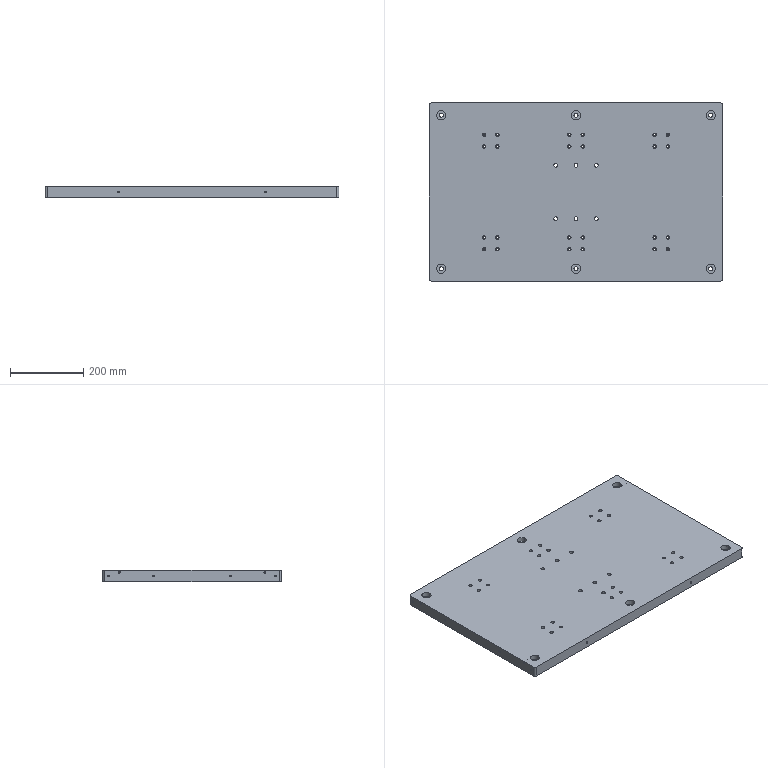NC program | Mastercam | posted with a generic post | part box 800 x 485 x 30 mm
Lines 631 to 1752 of 13355:
N6280 T20 M6
N6290 G0 G90 G17 G54 X332.781 Y6.265 A0. S5000 M3
N6300 G43 H20 Z50. M8
N6310 Z1.
N6320 G1 Z.533 F600.
N6330 Y17.265 Z.438 F4000.
N6340 Y28.265 Z.343
N6350 Y37.505 Z.264
N6360 X328.11 Y38.224 Z.249
N6370 X325. Y38.702 Z.221
N6380 X317.219 Y37.505 Z.154
N6390 Y36.679
N6400 Y25.679 Z.059
N6410 Y14.679 Z-.036
N6420 Y3.679 Z-.131
N6430 Y-.335 Z-.166
N6440 Y-7.321 Z-.226
N6450 Y-18.321 Z-.321
N6460 Y-29.321 Z-.416
N6470 Y-39.281 Z-.502
N6480 X321.887 Z-.511
N6490 X332.781 Z-.605
N6500 Y-37.758 Z-.606
N6510 Y-26.758 Z-.701
N6520 Y-15.758 Z-.796
N6530 Y-4.758 Z-.891
N6540 Y6.242 Z-.986
N6550 Y37.505
N6560 X325. Y38.702
N6570 X317.219 Y37.505
N6580 Y-.335
N6590 Y-39.281
N6600 X332.781
N6610 Y6.242
N6620 G2 X334.399 Y8.256 I2.063 J0.
N6630 G1 X344.186 Y10.416
N6640 G3 X345.804 Y12.43 I-.444 J2.014
N6650 G1 Y48.678
N6660 X325. Y51.878
N6670 X304.196 Y48.678
N6680 Y-.335
N6690 Y-52.304
N6700 X345.804
N6710 Y12.43
N6720 G2 X347.422 Y14.444 I2.063 J0.
N6730 G1 X357.209 Y16.603
N6740 G3 X358.827 Y18.617 I-.444 J2.014
N6750 G1 Y59.85
N6760 X325. Y65.054
N6770 X291.173 Y59.85
N6780 Y-.335
N6790 Y-65.327
N6800 X358.827
N6810 Y18.617
N6820 G2 X360.445 Y20.631 I2.063 J0.
N6830 G1 X370.232 Y22.791
N6840 G3 X371.85 Y24.805 I-.444 J2.014
N6850 G1 Y71.021
N6860 X325. Y78.231
N6870 X278.15 Y71.021
N6880 Y-.335
N6890 X278.151 Y-78.35
N6900 X371.849
N6910 X371.85 Y-78.347
N6920 Y24.805
N6930 G0 Z50.
N6940 X332.781 Y6.265
N6950 Z.014
N6960 G1 Z-.452 F600.
N6970 Y17.265 Z-.547 F4000.
N6980 Y28.265 Z-.642
N6990 Y37.505 Z-.722
N7000 X328.11 Y38.224 Z-.737
N7010 X325. Y38.702 Z-.764
N7020 X317.219 Y37.505 Z-.831
N7030 Y36.679 Z-.832
N7040 Y25.679 Z-.927
N7050 Y14.679 Z-1.022
N7060 Y3.679 Z-1.117
N7070 Y-.335 Z-1.152
N7080 Y-7.321 Z-1.212
N7090 Y-18.321 Z-1.307
N7100 Y-29.321 Z-1.402
N7110 Y-39.281 Z-1.488
N7120 X321.887 Z-1.497
N7130 X332.781 Z-1.591
N7140 Y-37.758 Z-1.592
N7150 Y-26.758 Z-1.687
N7160 Y-15.758 Z-1.782
N7170 Y-4.758 Z-1.876
N7180 Y6.242 Z-1.971
N7190 Y37.505
N7200 X325. Y38.702
N7210 X317.219 Y37.505
N7220 Y-.335
N7230 Y-39.281
N7240 X332.781
N7250 Y6.242
N7260 G2 X334.399 Y8.256 I2.063 J0.
N7270 G1 X344.186 Y10.416
N7280 G3 X345.804 Y12.43 I-.444 J2.014
N7290 G1 Y48.678
N7300 X325. Y51.878
N7310 X304.196 Y48.678
N7320 Y-.335
N7330 Y-52.304
N7340 X345.804
N7350 Y12.43
N7360 G2 X347.422 Y14.444 I2.063 J0.
N7370 G1 X357.209 Y16.603
N7380 G3 X358.827 Y18.617 I-.444 J2.014
N7390 G1 Y59.85
N7400 X325. Y65.054
N7410 X291.173 Y59.85
N7420 Y-.335
N7430 Y-65.327
N7440 X358.827
N7450 Y18.617
N7460 G2 X360.445 Y20.631 I2.063 J0.
N7470 G1 X370.232 Y22.791
N7480 G3 X371.85 Y24.805 I-.444 J2.014
N7490 G1 Y71.021
N7500 X325. Y78.231
N7510 X278.15 Y71.021
N7520 Y-.335
N7530 X278.151 Y-78.35
N7540 X371.849
N7550 X371.85 Y-78.347
N7560 Y24.805
N7570 G0 Z50.
N7580 X332.781 Y6.265
N7590 Z-.971
N7600 G1 Z-1.438 F600.
N7610 Y17.265 Z-1.533 F4000.
N7620 Y28.265 Z-1.628
N7630 Y37.505 Z-1.708
N7640 X328.11 Y38.224 Z-1.723
N7650 X325. Y38.702 Z-1.75
N7660 X317.219 Y37.505 Z-1.817
N7670 Y36.679 Z-1.818
N7680 Y25.679 Z-1.913
N7690 Y14.679 Z-2.008
N7700 Y3.679 Z-2.103
N7710 Y-.335 Z-2.137
N7720 Y-7.321 Z-2.198
N7730 Y-18.321 Z-2.293
N7740 Y-29.321 Z-2.388
N7750 Y-39.281 Z-2.473
N7760 X321.887 Z-2.482
N7770 X332.781 Z-2.576
N7780 Y-37.758 Z-2.577
N7790 Y-26.758 Z-2.672
N7800 Y-15.758 Z-2.767
N7810 Y-4.758 Z-2.862
N7820 Y6.242 Z-2.957
N7830 Y37.505
N7840 X325. Y38.702
N7850 X317.219 Y37.505
N7860 Y-.335
N7870 Y-39.281
N7880 X332.781
N7890 Y6.242
N7900 G2 X334.399 Y8.256 I2.063 J0.
N7910 G1 X344.186 Y10.416
N7920 G3 X345.804 Y12.43 I-.444 J2.014
N7930 G1 Y48.678
N7940 X325. Y51.878
N7950 X304.196 Y48.678
N7960 Y-.335
N7970 Y-52.304
N7980 X345.804
N7990 Y12.43
N8000 G2 X347.422 Y14.444 I2.063 J0.
N8010 G1 X357.209 Y16.603
N8020 G3 X358.827 Y18.617 I-.444 J2.014
N8030 G1 Y59.85
N8040 X325. Y65.054
N8050 X291.173 Y59.85
N8060 Y-.335
N8070 Y-65.327
N8080 X358.827
N8090 Y18.617
N8100 G2 X360.445 Y20.631 I2.063 J0.
N8110 G1 X370.232 Y22.791
N8120 G3 X371.85 Y24.805 I-.444 J2.014
N8130 G1 Y71.021
N8140 X325. Y78.231
N8150 X278.15 Y71.021
N8160 Y-.335
N8170 X278.151 Y-78.35
N8180 X371.849
N8190 X371.85 Y-78.347
N8200 Y24.805
N8210 G0 Z50.
N8220 X332.781 Y6.265
N8230 Z-1.957
N8240 G1 Z-2.424 F600.
N8250 Y17.265 Z-2.519 F4000.
N8260 Y28.265 Z-2.614
N8270 Y37.505 Z-2.693
N8280 X328.11 Y38.224 Z-2.709
N8290 X325. Y38.702 Z-2.736
N8300 X317.219 Y37.505 Z-2.803
N8310 Y36.679 Z-2.804
N8320 Y25.679 Z-2.899
N8330 Y14.679 Z-2.993
N8340 Y3.679 Z-3.088
N8350 Y-.335 Z-3.123
N8360 Y-7.321 Z-3.183
N8370 Y-18.321 Z-3.278
N8380 Y-29.321 Z-3.373
N8390 Y-39.281 Z-3.459
N8400 X321.887 Z-3.468
N8410 X332.781 Z-3.562
N8420 Y-37.758 Z-3.563
N8430 Y-26.758 Z-3.658
N8440 Y-15.758 Z-3.753
N8450 Y-4.758 Z-3.848
N8460 Y6.242 Z-3.943
N8470 Y37.505
N8480 X325. Y38.702
N8490 X317.219 Y37.505
N8500 Y-.335
N8510 Y-39.281
N8520 X332.781
N8530 Y6.242
N8540 G2 X334.399 Y8.256 I2.063 J0.
N8550 G1 X344.186 Y10.416
N8560 G3 X345.804 Y12.43 I-.444 J2.014
N8570 G1 Y48.678
N8580 X325. Y51.878
N8590 X304.196 Y48.678
N8600 Y-.335
N8610 Y-52.304
N8620 X345.804
N8630 Y12.43
N8640 G2 X347.422 Y14.444 I2.063 J0.
N8650 G1 X357.209 Y16.603
N8660 G3 X358.827 Y18.617 I-.444 J2.014
N8670 G1 Y59.85
N8680 X325. Y65.054
N8690 X291.173 Y59.85
N8700 Y-.335
N8710 Y-65.327
N8720 X358.827
N8730 Y18.617
N8740 G2 X360.445 Y20.631 I2.063 J0.
N8750 G1 X370.232 Y22.791
N8760 G3 X371.85 Y24.805 I-.444 J2.014
N8770 G1 Y71.021
N8780 X325. Y78.231
N8790 X278.15 Y71.021
N8800 Y-.335
N8810 X278.151 Y-78.35
N8820 X371.849
N8830 X371.85 Y-78.347
N8840 Y24.805
N8850 G0 Z50.
N8860 X332.781 Y6.265
N8870 Z-2.943
N8880 G1 Z-3.41 F600.
N8890 Y17.265 Z-3.504 F4000.
N8900 Y28.265 Z-3.599
N8910 Y37.505 Z-3.679
N8920 X328.11 Y38.224 Z-3.694
N8930 X325. Y38.702 Z-3.722
N8940 X317.219 Y37.505 Z-3.789
N8950 Y36.679
N8960 Y25.679 Z-3.884
N8970 Y14.679 Z-3.979
N8980 Y3.679 Z-4.074
N8990 Y-.335 Z-4.109
N9000 Y-7.321 Z-4.169
N9010 Y-18.321 Z-4.264
N9020 Y-29.321 Z-4.359
N9030 Y-39.281 Z-4.445
N9040 X321.887 Z-4.454
N9050 X332.781 Z-4.548
N9060 Y-37.758 Z-4.549
N9070 Y-26.758 Z-4.644
N9080 Y-15.758 Z-4.739
N9090 Y-4.758 Z-4.834
N9100 Y6.242 Z-4.929
N9110 Y37.505
N9120 X325. Y38.702
N9130 X317.219 Y37.505
N9140 Y-.335
N9150 Y-39.281
N9160 X332.781
N9170 Y6.242
N9180 G2 X334.399 Y8.256 I2.063 J0.
N9190 G1 X344.186 Y10.416
N9200 G3 X345.804 Y12.43 I-.444 J2.014
N9210 G1 Y48.678
N9220 X325. Y51.878
N9230 X304.196 Y48.678
N9240 Y-.335
N9250 Y-52.304
N9260 X345.804
N9270 Y12.43
N9280 G2 X347.422 Y14.444 I2.063 J0.
N9290 G1 X357.209 Y16.603
N9300 G3 X358.827 Y18.617 I-.444 J2.014
N9310 G1 Y59.85
N9320 X325. Y65.054
N9330 X291.173 Y59.85
N9340 Y-.335
N9350 Y-65.327
N9360 X358.827
N9370 Y18.617
N9380 G2 X360.445 Y20.631 I2.063 J0.
N9390 G1 X370.232 Y22.791
N9400 G3 X371.85 Y24.805 I-.444 J2.014
N9410 G1 Y71.021
N9420 X325. Y78.231
N9430 X278.15 Y71.021
N9440 Y-.335
N9450 X278.151 Y-78.35
N9460 X371.849
N9470 X371.85 Y-78.347
N9480 Y24.805
N9490 G0 Z50.
N9500 X332.781 Y6.265
N9510 Z-3.929
N9520 G1 Z-4.395 F600.
N9530 Y17.265 Z-4.49 F4000.
N9540 Y28.265 Z-4.585
N9550 Y37.505 Z-4.665
N9560 X328.11 Y38.224 Z-4.68
N9570 X325. Y38.702 Z-4.707
N9580 X317.219 Y37.505 Z-4.774
N9590 Y36.679 Z-4.775
N9600 Y25.679 Z-4.87
N9610 Y14.679 Z-4.965
N9620 Y3.679 Z-5.06
N9630 Y-.335 Z-5.094
N9640 Y-7.321 Z-5.155
N9650 Y-18.321 Z-5.25
N9660 Y-29.321 Z-5.345
N9670 Y-39.281 Z-5.431
N9680 X321.887 Z-5.44
N9690 X332.781 Z-5.534
N9700 Y-37.758 Z-5.535
N9710 Y-26.758 Z-5.629
N9720 Y-15.758 Z-5.724
N9730 Y-4.758 Z-5.819
N9740 Y6.242 Z-5.914
N9750 Y37.505
N9760 X325. Y38.702
N9770 X317.219 Y37.505
N9780 Y-.335
N9790 Y-39.281
N9800 X332.781
N9810 Y6.242
N9820 G2 X334.399 Y8.256 I2.063 J0.
N9830 G1 X344.186 Y10.416
N9840 G3 X345.804 Y12.43 I-.444 J2.014
N9850 G1 Y48.678
N9860 X325. Y51.878
N9870 X304.196 Y48.678
N9880 Y-.335
N9890 Y-52.304
N9900 X345.804
N9910 Y12.43
N9920 G2 X347.422 Y14.444 I2.063 J0.
N9930 G1 X357.209 Y16.603
N9940 G3 X358.827 Y18.617 I-.444 J2.014
N9950 G1 Y59.85
N9960 X325. Y65.054
N9970 X291.173 Y59.85
N9980 Y-.335
N9990 Y-65.327
N100 X358.827
N110 Y18.617
N120 G2 X360.445 Y20.631 I2.063 J0.
N130 G1 X370.232 Y22.791
N140 G3 X371.85 Y24.805 I-.444 J2.014
N150 G1 Y71.021
N160 X325. Y78.231
N170 X278.15 Y71.021
N180 Y-.335
N190 X278.151 Y-78.35
N200 X371.849
N210 X371.85 Y-78.347
N220 Y24.805
N230 G0 Z50.
N240 X332.781 Y6.265
N250 Z-4.914
N260 G1 Z-5.381 F600.
N270 Y17.265 Z-5.476 F4000.
N280 Y28.265 Z-5.571
N290 Y37.505 Z-5.651
N300 X328.11 Y38.224 Z-5.666
N310 X325. Y38.702 Z-5.693
N320 X317.219 Y37.505 Z-5.76
N330 Y36.679 Z-5.761
N340 Y25.679 Z-5.856
N350 Y14.679 Z-5.951
N360 Y3.679 Z-6.046
N370 Y-.335 Z-6.08
N380 Y-7.321 Z-6.14
N390 Y-18.321 Z-6.235
N400 Y-29.321 Z-6.33
N410 Y-39.281 Z-6.416
N420 X321.887 Z-6.425
N430 X332.781 Z-6.519
N440 Y-37.758 Z-6.52
N450 Y-26.758 Z-6.615
N460 Y-15.758 Z-6.71
N470 Y-4.758 Z-6.805
N480 Y6.242 Z-6.9
N490 Y37.505
N500 X325. Y38.702
N510 X317.219 Y37.505
N520 Y-.335
N530 Y-39.281
N540 X332.781
N550 Y6.242
N560 G2 X334.399 Y8.256 I2.063 J0.
N570 G1 X344.186 Y10.416
N580 G3 X345.804 Y12.43 I-.444 J2.014
N590 G1 Y48.678
N600 X325. Y51.878
N610 X304.196 Y48.678
N620 Y-.335
N630 Y-52.304
N640 X345.804
N650 Y12.43
N660 G2 X347.422 Y14.444 I2.063 J0.
N670 G1 X357.209 Y16.603
N680 G3 X358.827 Y18.617 I-.444 J2.014
N690 G1 Y59.85
N700 X325. Y65.054
N710 X291.173 Y59.85
N720 Y-.335
N730 Y-65.327
N740 X358.827
N750 Y18.617
N760 G2 X360.445 Y20.631 I2.063 J0.
N770 G1 X370.232 Y22.791
N780 G3 X371.85 Y24.805 I-.444 J2.014
N790 G1 Y71.021
N800 X325. Y78.231
N810 X278.15 Y71.021
N820 Y-.335
N830 X278.151 Y-78.35
N840 X371.849
N850 X371.85 Y-78.347
N860 Y24.805
N870 G0 Z50.
N880 X202.781 Y6.265
N890 Z1.
N900 G1 Z.533 F600.
N910 Y17.265 Z.438 F4000.
N920 Y28.265 Z.343
N930 Y37.505 Z.264
N940 X198.11 Y38.224 Z.249
N950 X195. Y38.702 Z.221
N960 X187.219 Y37.505 Z.154
N970 Y36.679
N980 Y25.679 Z.059
N990 Y14.679 Z-.036
N1000 Y3.679 Z-.131
N1010 Y-7.321 Z-.226
N1020 Y-18.321 Z-.321
N1030 Y-29.321 Z-.416
N1040 Y-39.281 Z-.502
N1050 X191.887 Z-.511
N1060 X202.781 Z-.605
N1070 Y-37.758 Z-.606
N1080 Y-26.758 Z-.701
N1090 Y-15.758 Z-.796
N1100 Y-4.758 Z-.891
N1110 Y-.335 Z-.929
N1120 Y6.242 Z-.986
N1130 Y37.505
N1140 X195. Y38.702
N1150 X187.219 Y37.505
N1160 Y-39.281
N1170 X202.781
N1180 Y-.335
N1190 Y6.242
N1200 G2 X204.399 Y8.256 I2.063 J0.
N1210 G1 X214.186 Y10.416
N1220 G3 X215.804 Y12.43 I-.444 J2.014
N1230 G1 Y48.678
N1240 X195. Y51.878
N1250 X174.196 Y48.678
N1260 Y-52.304
N1270 X215.804
N1280 Y-.335
N1290 Y12.43
N1300 G2 X217.422 Y14.444 I2.063 J0.
N1310 G1 X227.209 Y16.603
N1320 G3 X228.827 Y18.617 I-.444 J2.014
N1330 G1 Y59.85
N1340 X195. Y65.054
N1350 X161.173 Y59.85
N1360 Y-65.327
N1370 X228.827
N1380 Y-.335
N1390 Y18.617
N1400 G2 X230.445 Y20.631 I2.063 J0.
N1410 G1 X240.232 Y22.791
N1420 G3 X241.85 Y24.805 I-.444 J2.014
N1430 G1 Y71.021
N1440 X195. Y78.231
N1450 X148.15 Y71.021
N1460 Y-78.347
N1470 X148.151 Y-78.35
N1480 X241.849
N1490 X241.85 Y-.335
N1500 Y24.805
N1510 G0 Z50.
N1520 X202.781 Y6.265
N1530 Z.014
N1540 G1 Z-.452 F600.
N1550 Y17.265 Z-.547 F4000.
N1560 Y28.265 Z-.642
N1570 Y37.505 Z-.722
N1580 X198.11 Y38.224 Z-.737
N1590 X195. Y38.702 Z-.764
N1600 X187.219 Y37.505 Z-.831
N1610 Y36.679 Z-.832
N1620 Y25.679 Z-.927
N1630 Y14.679 Z-1.022
N1640 Y3.679 Z-1.117
N1650 Y-7.321 Z-1.212
N1660 Y-18.321 Z-1.307
N1670 Y-29.321 Z-1.402
N1680 Y-39.281 Z-1.488
N1690 X191.887 Z-1.497
N1700 X202.781 Z-1.591
N1710 Y-37.758 Z-1.592
N1720 Y-26.758 Z-1.687
N1730 Y-15.758 Z-1.782
N1740 Y-4.758 Z-1.876
N1750 Y-.335 Z-1.915
N1760 Y6.242 Z-1.971
N1770 Y37.505
N1780 X195. Y38.702
N1790 X187.219 Y37.505
N1800 Y-39.281
N1810 X202.781
N1820 Y-.335
N1830 Y6.242
N1840 G2 X204.399 Y8.256 I2.063 J0.
N1850 G1 X214.186 Y10.416
N1860 G3 X215.804 Y12.43 I-.444 J2.014
N1870 G1 Y48.678
N1880 X195. Y51.878
N1890 X174.196 Y48.678
N1900 Y-52.304
N1910 X215.804
N1920 Y-.335
N1930 Y12.43
N1940 G2 X217.422 Y14.444 I2.063 J0.
N1950 G1 X227.209 Y16.603
N1960 G3 X228.827 Y18.617 I-.444 J2.014
N1970 G1 Y59.85
N1980 X195. Y65.054
N1990 X161.173 Y59.85
N2000 Y-65.327
N2010 X228.827
N2020 Y-.335
N2030 Y18.617
N2040 G2 X230.445 Y20.631 I2.063 J0.
N2050 G1 X240.232 Y22.791
N2060 G3 X241.85 Y24.805 I-.444 J2.014
N2070 G1 Y71.021
N2080 X195. Y78.231
N2090 X148.15 Y71.021
N2100 Y-78.347
N2110 X148.151 Y-78.35
N2120 X241.849
N2130 X241.85 Y-.335
N2140 Y24.805
N2150 G0 Z50.
N2160 X202.781 Y6.265
N2170 Z-.971
N2180 G1 Z-1.438 F600.
N2190 Y17.265 Z-1.533 F4000.
N2200 Y28.265 Z-1.628
N2210 Y37.505 Z-1.708
N2220 X198.11 Y38.224 Z-1.723
N2230 X195. Y38.702 Z-1.75
N2240 X187.219 Y37.505 Z-1.817
N2250 Y36.679 Z-1.818
N2260 Y25.679 Z-1.913
N2270 Y14.679 Z-2.008
N2280 Y3.679 Z-2.103
N2290 Y-7.321 Z-2.198
N2300 Y-18.321 Z-2.293
N2310 Y-29.321 Z-2.388
N2320 Y-39.281 Z-2.473
N2330 X191.887 Z-2.482
N2340 X202.781 Z-2.576
N2350 Y-37.758 Z-2.577
N2360 Y-26.758 Z-2.672
N2370 Y-15.758 Z-2.767
N2380 Y-4.758 Z-2.862
N2390 Y-.335 Z-2.9
N2400 Y6.242 Z-2.957
N2410 Y37.505
N2420 X195. Y38.702
N2430 X187.219 Y37.505
N2440 Y-39.281
N2450 X202.781
N2460 Y-.335
N2470 Y6.242
N2480 G2 X204.399 Y8.256 I2.063 J0.
N2490 G1 X214.186 Y10.416
N2500 G3 X215.804 Y12.43 I-.444 J2.014
N2510 G1 Y48.678
N2520 X195. Y51.878
N2530 X174.196 Y48.678
N2540 Y-52.304
N2550 X215.804
N2560 Y-.335
N2570 Y12.43
N2580 G2 X217.422 Y14.444 I2.063 J0.
N2590 G1 X227.209 Y16.603
N2600 G3 X228.827 Y18.617 I-.444 J2.014
N2610 G1 Y59.85
N2620 X195. Y65.054
N2630 X161.173 Y59.85
N2640 Y-65.327
N2650 X228.827
N2660 Y-.335
N2670 Y18.617
N2680 G2 X230.445 Y20.631 I2.063 J0.
N2690 G1 X240.232 Y22.791
N2700 G3 X241.85 Y24.805 I-.444 J2.014
N2710 G1 Y71.021
N2720 X195. Y78.231
N2730 X148.15 Y71.021
N2740 Y-78.347
N2750 X148.151 Y-78.35
N2760 X241.849
N2770 X241.85 Y-.335
N2780 Y24.805
N2790 G0 Z50.
N2800 X202.781 Y6.265
N2810 Z-1.957
N2820 G1 Z-2.424 F600.
N2830 Y17.265 Z-2.519 F4000.
N2840 Y28.265 Z-2.614
N2850 Y37.505 Z-2.693
N2860 X198.11 Y38.224 Z-2.709
N2870 X195. Y38.702 Z-2.736
N2880 X187.219 Y37.505 Z-2.803
N2890 Y36.679 Z-2.804
N2900 Y25.679 Z-2.899
N2910 Y14.679 Z-2.993
N2920 Y3.679 Z-3.088
N2930 Y-7.321 Z-3.183
N2940 Y-18.321 Z-3.278
N2950 Y-29.321 Z-3.373
N2960 Y-39.281 Z-3.459
N2970 X191.887 Z-3.468
N2980 X202.781 Z-3.562
N2990 Y-37.758 Z-3.563
N3000 Y-26.758 Z-3.658
N3010 Y-15.758 Z-3.753
N3020 Y-4.758 Z-3.848
N3030 Y-.335 Z-3.886
N3040 Y6.242 Z-3.943
N3050 Y37.505
N3060 X195. Y38.702
N3070 X187.219 Y37.505
N3080 Y-39.281
N3090 X202.781
N3100 Y-.335
N3110 Y6.242
N3120 G2 X204.399 Y8.256 I2.063 J0.
N3130 G1 X214.186 Y10.416
N3140 G3 X215.804 Y12.43 I-.444 J2.014
N3150 G1 Y48.678
N3160 X195. Y51.878
N3170 X174.196 Y48.678
N3180 Y-52.304
N3190 X215.804
N3200 Y-.335
N3210 Y12.43
N3220 G2 X217.422 Y14.444 I2.063 J0.
N3230 G1 X227.209 Y16.603
N3240 G3 X228.827 Y18.617 I-.444 J2.014
N3250 G1 Y59.85
N3260 X195. Y65.054
N3270 X161.173 Y59.85
N3280 Y-65.327
N3290 X228.827
N3300 Y-.335
N3310 Y18.617
N3320 G2 X230.445 Y20.631 I2.063 J0.
N3330 G1 X240.232 Y22.791
N3340 G3 X241.85 Y24.805 I-.444 J2.014
N3350 G1 Y71.021
N3360 X195. Y78.231
N3370 X148.15 Y71.021
N3380 Y-78.347
N3390 X148.151 Y-78.35
N3400 X241.849
N3410 X241.85 Y-.335
N3420 Y24.805
N3430 G0 Z50.
N3440 X202.781 Y6.265
N3450 Z-2.943
N3460 G1 Z-3.41 F600.
N3470 Y17.265 Z-3.504 F4000.
N3480 Y28.265 Z-3.599
N3490 Y37.505 Z-3.679
N3500 X198.11 Y38.224 Z-3.694
N3510 X195. Y38.702 Z-3.722
N3520 X187.219 Y37.505 Z-3.789
N3530 Y36.679
N3540 Y25.679 Z-3.884
N3550 Y14.679 Z-3.979
N3560 Y3.679 Z-4.074
N3570 Y-7.321 Z-4.169
N3580 Y-18.321 Z-4.264
N3590 Y-29.321 Z-4.359
N3600 Y-39.281 Z-4.445
N3610 X191.887 Z-4.454
N3620 X202.781 Z-4.548
N3630 Y-37.758 Z-4.549
N3640 Y-26.758 Z-4.644
N3650 Y-15.758 Z-4.739
N3660 Y-4.758 Z-4.834
N3670 Y-.335 Z-4.872
N3680 Y6.242 Z-4.929
N3690 Y37.505
N3700 X195. Y38.702
N3710 X187.219 Y37.505
N3720 Y-39.281
N3730 X202.781
N3740 Y-.335
N3750 Y6.242
N3760 G2 X204.399 Y8.256 I2.063 J0.
N3770 G1 X214.186 Y10.416
N3780 G3 X215.804 Y12.43 I-.444 J2.014
N3790 G1 Y48.678
N3800 X195. Y51.878
N3810 X174.196 Y48.678
N3820 Y-52.304
N3830 X215.804
N3840 Y-.335
N3850 Y12.43
N3860 G2 X217.422 Y14.444 I2.063 J0.
N3870 G1 X227.209 Y16.603
N3880 G3 X228.827 Y18.617 I-.444 J2.014
N3890 G1 Y59.85
N3900 X195. Y65.054
N3910 X161.173 Y59.85
N3920 Y-65.327
N3930 X228.827
N3940 Y-.335
N3950 Y18.617
N3960 G2 X230.445 Y20.631 I2.063 J0.
N3970 G1 X240.232 Y22.791
N3980 G3 X241.85 Y24.805 I-.444 J2.014
N3990 G1 Y71.021
N4000 X195. Y78.231
N4010 X148.15 Y71.021
N4020 Y-78.347
N4030 X148.151 Y-78.35
N4040 X241.849
N4050 X241.85 Y-.335
N4060 Y24.805
N4070 G0 Z50.
N4080 X202.781 Y6.265
N4090 Z-3.929
N4100 G1 Z-4.395 F600.
N4110 Y17.265 Z-4.49 F4000.
N4120 Y28.265 Z-4.585
N4130 Y37.505 Z-4.665
N4140 X198.11 Y38.224 Z-4.68
N4150 X195. Y38.702 Z-4.707
N4160 X187.219 Y37.505 Z-4.774
N4170 Y36.679 Z-4.775
N4180 Y25.679 Z-4.87
N4190 Y14.679 Z-4.965
N4200 Y3.679 Z-5.06
N4210 Y-7.321 Z-5.155
N4220 Y-18.321 Z-5.25
N4230 Y-29.321 Z-5.345
N4240 Y-39.281 Z-5.431
N4250 X191.887 Z-5.44
N4260 X202.781 Z-5.534
N4270 Y-37.758 Z-5.535
N4280 Y-26.758 Z-5.629
N4290 Y-15.758 Z-5.724
N4300 Y-4.758 Z-5.819
N4310 Y-.335 Z-5.858
N4320 Y6.242 Z-5.914
N4330 Y37.505
N4340 X195. Y38.702
N4350 X187.219 Y37.505
N4360 Y-39.281
N4370 X202.781
N4380 Y-.335
N4390 Y6.242
N4400 G2 X204.399 Y8.256 I2.063 J0.
N4410 G1 X214.186 Y10.416
N4420 G3 X215.804 Y12.43 I-.444 J2.014
N4430 G1 Y48.678
N4440 X195. Y51.878
N4450 X174.196 Y48.678
N4460 Y-52.304
N4470 X215.804
N4480 Y-.335
N4490 Y12.43
N4500 G2 X217.422 Y14.444 I2.063 J0.
N4510 G1 X227.209 Y16.603
N4520 G3 X228.827 Y18.617 I-.444 J2.014
N4530 G1 Y59.85
N4540 X195. Y65.054
N4550 X161.173 Y59.85
N4560 Y-65.327
N4570 X228.827
N4580 Y-.335
N4590 Y18.617
N4600 G2 X230.445 Y20.631 I2.063 J0.
N4610 G1 X240.232 Y22.791
N4620 G3 X241.85 Y24.805 I-.444 J2.014
N4630 G1 Y71.021
N4640 X195. Y78.231
N4650 X148.15 Y71.021
N4660 Y-78.347
N4670 X148.151 Y-78.35
N4680 X241.849
N4690 X241.85 Y-.335
N4700 Y24.805
N4710 G0 Z50.
N4720 X202.781 Y6.265
N4730 Z-4.914
N4740 G1 Z-5.381 F600.
N4750 Y17.265 Z-5.476 F4000.
N4760 Y28.265 Z-5.571
N4770 Y37.505 Z-5.651
N4780 X198.11 Y38.224 Z-5.666
N4790 X195. Y38.702 Z-5.693
N4800 X187.219 Y37.505 Z-5.76
N4810 Y36.679 Z-5.761
N4820 Y25.679 Z-5.856
N4830 Y14.679 Z-5.951
N4840 Y3.679 Z-6.046
N4850 Y-7.321 Z-6.14
N4860 Y-18.321 Z-6.235
N4870 Y-29.321 Z-6.33
N4880 Y-39.281 Z-6.416
N4890 X191.887 Z-6.425
N4900 X202.781 Z-6.519
N4910 Y-37.758 Z-6.52
N4920 Y-26.758 Z-6.615
N4930 Y-15.758 Z-6.71
N4940 Y-4.758 Z-6.805
N4950 Y-.335 Z-6.843
N4960 Y6.242 Z-6.9
N4970 Y37.505
N4980 X195. Y38.702
N4990 X187.219 Y37.505
N5000 Y-39.281
N5010 X202.781
N5020 Y-.335
N5030 Y6.242
N5040 G2 X204.399 Y8.256 I2.063 J0.
N5050 G1 X214.186 Y10.416
N5060 G3 X215.804 Y12.43 I-.444 J2.014
N5070 G1 Y48.678
N5080 X195. Y51.878
N5090 X174.196 Y48.678
N5100 Y-52.304
N5110 X215.804
N5120 Y-.335
N5130 Y12.43
N5140 G2 X217.422 Y14.444 I2.063 J0.
N5150 G1 X227.209 Y16.603
N5160 G3 X228.827 Y18.617 I-.444 J2.014
N5170 G1 Y59.85
N5180 X195. Y65.054
N5190 X161.173 Y59.85
N5200 Y-65.327
N5210 X228.827
N5220 Y-.335
N5230 Y18.617
N5240 G2 X230.445 Y20.631 I2.063 J0.
N5250 G1 X240.232 Y22.791
N5260 G3 X241.85 Y24.805 I-.444 J2.014
N5270 G1 Y71.021
N5280 X195. Y78.231
N5290 X148.15 Y71.021
N5300 Y-78.347
N5310 X148.151 Y-78.35
N5320 X241.849
N5330 X241.85 Y-.335
N5340 Y24.805
N5350 G0 Z50.
N5360 X72.781 Y6.265
N5370 Z1.
N5380 G1 Z.533 F600.
N5390 Y17.265 Z.438 F4000.
N5400 Y28.265 Z.343
N5410 Y37.505 Z.264
N5420 X68.11 Y38.224 Z.249
N5430 X65. Y38.702 Z.221
N5440 X57.219 Y37.505 Z.154
N5450 Y36.679
N5460 Y25.679 Z.059
N5470 Y14.679 Z-.036
N5480 Y3.679 Z-.131
N5490 Y-7.321 Z-.226
N5500 Y-18.321 Z-.321
N5510 Y-29.321 Z-.416
N5520 Y-39.281 Z-.502
N5530 X61.887 Z-.511
N5540 X72.781 Z-.605
N5550 Y-37.758 Z-.606
N5560 Y-26.758 Z-.701
N5570 Y-15.758 Z-.796
N5580 Y-4.758 Z-.891
N5590 Y-.335 Z-.929
N5600 Y6.242 Z-.986
N5610 Y37.505
N5620 X65. Y38.702
N5630 X57.219 Y37.505
N5640 Y-39.281
N5650 X72.781
N5660 Y-.335
N5670 Y6.242
N5680 G2 X74.399 Y8.256 I2.063 J0.
N5690 G1 X84.186 Y10.416
N5700 G3 X85.804 Y12.43 I-.444 J2.014
N5710 G1 Y48.678
N5720 X65. Y51.878
N5730 X44.196 Y48.678
N5740 Y-52.304
N5750 X85.804
N5760 Y-.335
N5770 Y12.43
N5780 G2 X87.422 Y14.444 I2.063 J0.
N5790 G1 X97.209 Y16.603
N5800 G3 X98.827 Y18.617 I-.444 J2.014
N5810 G1 Y59.85
N5820 X65. Y65.054
N5830 X31.173 Y59.85
N5840 Y-65.327
N5850 X98.827
N5860 Y-.335
N5870 Y18.617
N5880 G2 X100.445 Y20.631 I2.063 J0.
N5890 G1 X110.232 Y22.791
N5900 G3 X111.85 Y24.805 I-.444 J2.014
N5910 G1 Y71.021
N5920 X65. Y78.231
N5930 X18.15 Y71.021
N5940 Y-78.347
N5950 X18.151 Y-78.35
N5960 X111.849
N5970 X111.85 Y-.335
N5980 Y24.805
N5990 G0 Z50.
N6000 X72.781 Y6.265
N6010 Z.014
N6020 G1 Z-.452 F600.
N6030 Y17.265 Z-.547 F4000.
N6040 Y28.265 Z-.642
N6050 Y37.505 Z-.722
N6060 X68.11 Y38.224 Z-.737
N6070 X65. Y38.702 Z-.764
N6080 X57.219 Y37.505 Z-.831
N6090 Y36.679 Z-.832
N6100 Y25.679 Z-.927
N6110 Y14.679 Z-1.022
N6120 Y3.679 Z-1.117
N6130 Y-7.321 Z-1.212
N6140 Y-18.321 Z-1.307
N6150 Y-29.321 Z-1.402
N6160 Y-39.281 Z-1.488
N6170 X61.887 Z-1.497
N6180 X72.781 Z-1.591
N6190 Y-37.758 Z-1.592
N6200 Y-26.758 Z-1.687
N6210 Y-15.758 Z-1.782
N6220 Y-4.758 Z-1.876
N6230 Y-.335 Z-1.915
N6240 Y6.242 Z-1.971
N6250 Y37.505
N6260 X65. Y38.702
N6270 X57.219 Y37.505
N6280 Y-39.281
N6290 X72.781
N6300 Y-.335
N6310 Y6.242
N6320 G2 X74.399 Y8.256 I2.063 J0.
N6330 G1 X84.186 Y10.416
N6340 G3 X85.804 Y12.43 I-.444 J2.014
N6350 G1 Y48.678
N6360 X65. Y51.878
N6370 X44.196 Y48.678
N6380 Y-52.304
N6390 X85.804
N6400 Y-.335
N6410 Y12.43
N6420 G2 X87.422 Y14.444 I2.063 J0.
N6430 G1 X97.209 Y16.603
N6440 G3 X98.827 Y18.617 I-.444 J2.014
N6450 G1 Y59.85
N6460 X65. Y65.054
N6470 X31.173 Y59.85
N6480 Y-65.327
N6490 X98.827
N6500 Y-.335
N6510 Y18.617
N6520 G2 X100.445 Y20.631 I2.063 J0.
N6530 G1 X110.232 Y22.791
N6540 G3 X111.85 Y24.805 I-.444 J2.014
N6550 G1 Y71.021
N6560 X65. Y78.231
N6570 X18.15 Y71.021
N6580 Y-78.347
N6590 X18.151 Y-78.35
N6600 X111.849
N6610 X111.85 Y-.335
N6620 Y24.805
N6630 G0 Z50.
N6640 X72.781 Y6.265
N6650 Z-.971
N6660 G1 Z-1.438 F600.
N6670 Y17.265 Z-1.533 F4000.
N6680 Y28.265 Z-1.628
N6690 Y37.505 Z-1.708
N6700 X68.11 Y38.224 Z-1.723
N6710 X65. Y38.702 Z-1.75
N6720 X57.219 Y37.505 Z-1.817
N6730 Y36.679 Z-1.818
N6740 Y25.679 Z-1.913
N6750 Y14.679 Z-2.008
N6760 Y3.679 Z-2.103
N6770 Y-7.321 Z-2.198
N6780 Y-18.321 Z-2.293
N6790 Y-29.321 Z-2.388
N6800 Y-39.281 Z-2.473
N6810 X61.887 Z-2.482
N6820 X72.781 Z-2.576
N6830 Y-37.758 Z-2.577
N6840 Y-26.758 Z-2.672
N6850 Y-15.758 Z-2.767
N6860 Y-4.758 Z-2.862
N6870 Y-.335 Z-2.9
N6880 Y6.242 Z-2.957
N6890 Y37.505
N6900 X65. Y38.702
N6910 X57.219 Y37.505
N6920 Y-39.281
N6930 X72.781
N6940 Y-.335
N6950 Y6.242
N6960 G2 X74.399 Y8.256 I2.063 J0.
N6970 G1 X84.186 Y10.416
N6980 G3 X85.804 Y12.43 I-.444 J2.014
N6990 G1 Y48.678
N7000 X65. Y51.878
N7010 X44.196 Y48.678
N7020 Y-52.304
N7030 X85.804
N7040 Y-.335
N7050 Y12.43
N7060 G2 X87.422 Y14.444 I2.063 J0.
N7070 G1 X97.209 Y16.603
N7080 G3 X98.827 Y18.617 I-.444 J2.014
N7090 G1 Y59.85
N7100 X65. Y65.054
N7110 X31.173 Y59.85
N7120 Y-65.327
N7130 X98.827
N7140 Y-.335
N7150 Y18.617
N7160 G2 X100.445 Y20.631 I2.063 J0.
N7170 G1 X110.232 Y22.791
N7180 G3 X111.85 Y24.805 I-.444 J2.014
N7190 G1 Y71.021
N7200 X65. Y78.231
N7210 X18.15 Y71.021
N7220 Y-78.347
N7230 X18.151 Y-78.35
N7240 X111.849
N7250 X111.85 Y-.335
N7260 Y24.805
N7270 G0 Z50.
N7280 X72.781 Y6.265
N7290 Z-1.957
N7300 G1 Z-2.424 F600.
N7310 Y17.265 Z-2.519 F4000.
N7320 Y28.265 Z-2.614
N7330 Y37.505 Z-2.693
N7340 X68.11 Y38.224 Z-2.709
N7350 X65. Y38.702 Z-2.736
N7360 X57.219 Y37.505 Z-2.803
N7370 Y36.679 Z-2.804
N7380 Y25.679 Z-2.899
N7390 Y14.679 Z-2.993
N7400 Y3.679 Z-3.088
N7410 Y-7.321 Z-3.183
N7420 Y-18.321 Z-3.278
N7430 Y-29.321 Z-3.373
N7440 Y-39.281 Z-3.459
N7450 X61.887 Z-3.468
N7460 X72.781 Z-3.562
N7470 Y-37.758 Z-3.563
N7480 Y-26.758 Z-3.658
N7490 Y-15.758 Z-3.753
N7500 Y-4.758 Z-3.848
N7510 Y-.335 Z-3.886
N7520 Y6.242 Z-3.943
N7530 Y37.505
N7540 X65. Y38.702
N7550 X57.219 Y37.505
N7560 Y-39.281
N7570 X72.781
N7580 Y-.335
N7590 Y6.242